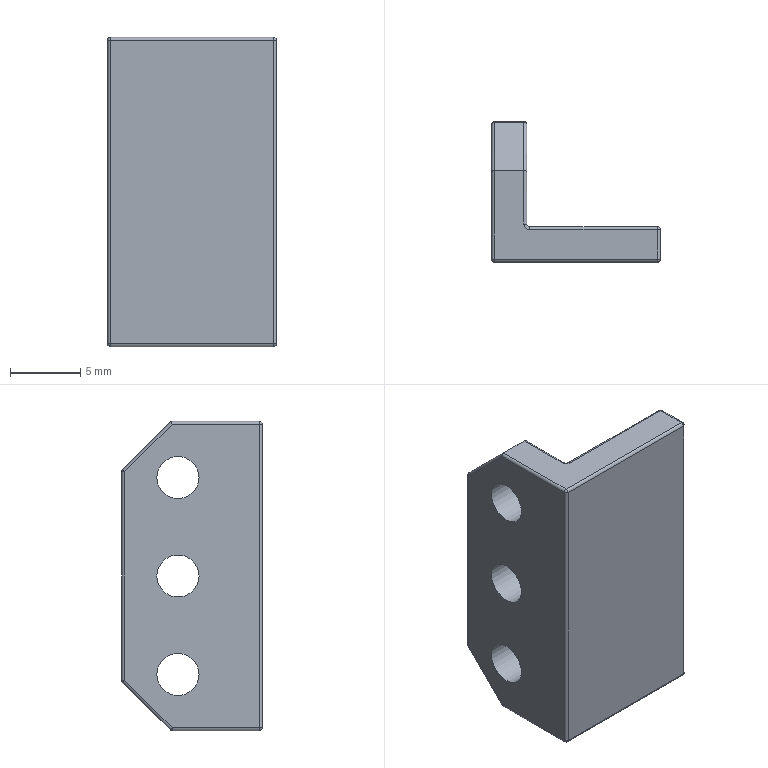Part | STEP file | 1-53.2 | 1 solid | 50 faces | box 12 x 10 x 22 mm | volume 987.448 mm3 | cylinder 26 | sphere 12 | plane 10 | torus 2 | commonest cylinder face diameters 0.4 x23 3 x3